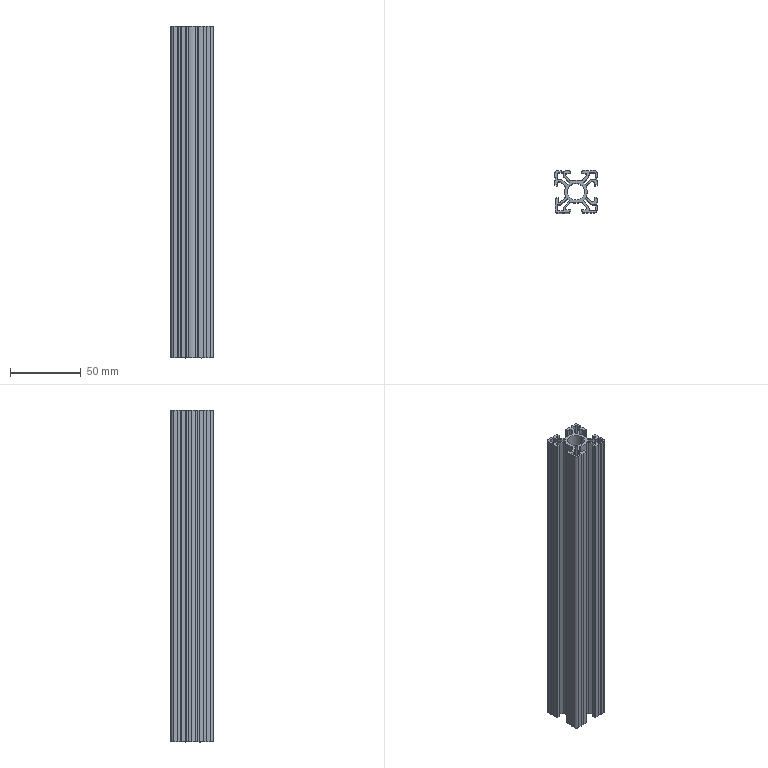Part | STEP file | 3030 printer curtain rod | 1 solid | 154 faces | box 29.915 x 30.09 x 235 mm | volume 73681 mm3 | plane 110 | cylinder 44 | commonest cylinder face diameters 2 x15 4 x14 5 x8 16 x5 12 x2